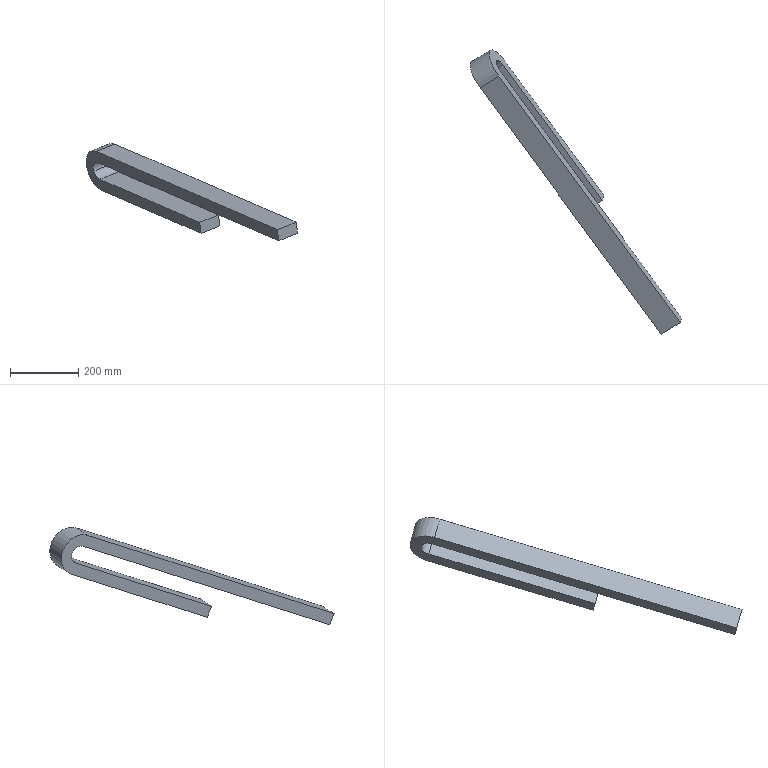Part | SolidWorks | features ExtruThin 1 | 1 solid | 12 faces | box 617.546 x 830.514 x 284.328 mm | volume 3734019 mm3 | plane 8 | cylinder 4 | commonest cylinder face diameters 54 x2 124 x2
STEP:
#1=CARTESIAN_POINT('',(136.827,-667.539,2230.426));
#2=VERTEX_POINT('',#1);
#3=CARTESIAN_POINT('',(147.549,-700.908,2255.142));
#4=VERTEX_POINT('',#3);
#5=CARTESIAN_POINT('',(150.913,-690.573,2230.426));
#6=DIRECTION('',(0.8091,0.4948,0.317));
#7=DIRECTION('',(-0.1246,-0.3828,0.9154));
#8=AXIS2_PLACEMENT_3D('',#5,#6,#7);
#9=CIRCLE('',#8,27.);
#10=EDGE_CURVE('',#2,#4,#9,.T.);
#11=ORIENTED_EDGE('',*,*,#10,.F.);
#12=CARTESIAN_POINT('',(191.847,-633.893,2251.985));
#13=VERTEX_POINT('',#12);
#14=CARTESIAN_POINT('',(136.827,-667.539,2230.426));
#15=DIRECTION('',(0.8091,0.4948,0.317));
#16=VECTOR('',#15,1000.);
#17=LINE('',#14,#16);
#18=EDGE_CURVE('',#2,#13,#17,.T.);
#19=ORIENTED_EDGE('',*,*,#18,.T.);
#20=CARTESIAN_POINT('',(202.568,-667.262,2276.7));
#21=VERTEX_POINT('',#20);
#22=CARTESIAN_POINT('',(205.933,-656.927,2251.985));
#23=DIRECTION('',(0.8091,0.4948,0.317));
#24=DIRECTION('',(-0.1246,-0.3828,0.9154));
#25=AXIS2_PLACEMENT_3D('',#22,#23,#24);
#26=CIRCLE('',#25,27.);
#27=EDGE_CURVE('',#13,#21,#26,.T.);
#28=ORIENTED_EDGE('',*,*,#27,.T.);
#29=CARTESIAN_POINT('',(147.549,-700.908,2255.142));
#30=DIRECTION('',(0.8091,0.4948,0.317));
#31=VECTOR('',#30,1000.);
#32=LINE('',#29,#31);
#33=EDGE_CURVE('',#4,#21,#32,.T.);
#34=ORIENTED_EDGE('',*,*,#33,.F.);
#35=EDGE_LOOP('',(#11,#19,#28,#34));
#36=FACE_OUTER_BOUND('',#35,.T.);
#37=CARTESIAN_POINT('',(150.913,-690.573,2230.426));
#38=DIRECTION('',(0.8091,0.4948,0.317));
#39=DIRECTION('',(-0.5217,0.8531,0.));
#40=AXIS2_PLACEMENT_3D('',#37,#38,#39);
#41=CYLINDRICAL_SURFACE('',#40,27.);
#42=ADVANCED_FACE('',(#36),#41,.F.);
#43=CARTESIAN_POINT('',(158.639,-666.841,2173.671));
#44=VERTEX_POINT('',#43);
#45=CARTESIAN_POINT('',(118.567,-637.68,2230.426));
#46=VERTEX_POINT('',#45);
#47=CARTESIAN_POINT('',(150.913,-690.573,2230.426));
#48=DIRECTION('',(0.8091,0.4948,0.317));
#49=DIRECTION('',(-0.5217,0.8531,0.));
#50=AXIS2_PLACEMENT_3D('',#47,#48,#49);
#51=CIRCLE('',#50,62.);
#52=EDGE_CURVE('',#44,#46,#51,.T.);
#53=ORIENTED_EDGE('',*,*,#52,.T.);
#54=CARTESIAN_POINT('',(173.587,-604.034,2251.985));
#55=VERTEX_POINT('',#54);
#56=CARTESIAN_POINT('',(118.567,-637.68,2230.426));
#57=DIRECTION('',(0.8091,0.4948,0.317));
#58=VECTOR('',#57,1000.);
#59=LINE('',#56,#58);
#60=EDGE_CURVE('',#46,#55,#59,.T.);
#61=ORIENTED_EDGE('',*,*,#60,.T.);
#62=CARTESIAN_POINT('',(213.659,-633.195,2195.23));
#63=VERTEX_POINT('',#62);
#64=CARTESIAN_POINT('',(205.933,-656.927,2251.985));
#65=DIRECTION('',(0.8091,0.4948,0.317));
#66=DIRECTION('',(-0.5217,0.8531,0.));
#67=AXIS2_PLACEMENT_3D('',#64,#65,#66);
#68=CIRCLE('',#67,62.);
#69=EDGE_CURVE('',#63,#55,#68,.T.);
#70=ORIENTED_EDGE('',*,*,#69,.F.);
#71=CARTESIAN_POINT('',(158.639,-666.841,2173.671));
#72=DIRECTION('',(0.8091,0.4948,0.317));
#73=VECTOR('',#72,1000.);
#74=LINE('',#71,#73);
#75=EDGE_CURVE('',#44,#63,#74,.T.);
#76=ORIENTED_EDGE('',*,*,#75,.F.);
#77=EDGE_LOOP('',(#53,#61,#70,#76));
#78=FACE_OUTER_BOUND('',#77,.T.);
#79=CARTESIAN_POINT('',(150.913,-690.573,2230.426));
#80=DIRECTION('',(0.8091,0.4948,0.317));
#81=DIRECTION('',(-0.5217,0.8531,0.));
#82=AXIS2_PLACEMENT_3D('',#79,#80,#81);
#83=CYLINDRICAL_SURFACE('',#82,62.);
#84=ADVANCED_FACE('',(#78),#83,.T.);
#85=CARTESIAN_POINT('',(198.207,-680.659,2308.739));
#86=VERTEX_POINT('',#85);
#87=CARTESIAN_POINT('',(727.663,-1399.917,2080.056));
#88=VERTEX_POINT('',#87);
#89=CARTESIAN_POINT('',(727.663,-1399.917,2080.056));
#90=DIRECTION('',(0.5743,-0.7802,-0.248));
#91=VECTOR('',#90,1000.);
#92=LINE('',#89,#91);
#93=EDGE_CURVE('',#86,#88,#92,.T.);
#94=ORIENTED_EDGE('',*,*,#93,.F.);
#95=CARTESIAN_POINT('',(143.187,-714.305,2287.181));
#96=VERTEX_POINT('',#95);
#97=CARTESIAN_POINT('',(143.187,-714.305,2287.181));
#98=DIRECTION('',(0.8091,0.4948,0.317));
#99=VECTOR('',#98,1000.);
#100=LINE('',#97,#99);
#101=EDGE_CURVE('',#96,#86,#100,.T.);
#102=ORIENTED_EDGE('',*,*,#101,.F.);
#103=CARTESIAN_POINT('',(672.643,-1433.563,2058.497));
#104=VERTEX_POINT('',#103);
#105=CARTESIAN_POINT('',(672.643,-1433.563,2058.497));
#106=DIRECTION('',(0.5743,-0.7802,-0.248));
#107=VECTOR('',#106,1000.);
#108=LINE('',#105,#107);
#109=EDGE_CURVE('',#96,#104,#108,.T.);
#110=ORIENTED_EDGE('',*,*,#109,.T.);
#111=CARTESIAN_POINT('',(672.643,-1433.563,2058.497));
#112=DIRECTION('',(0.8091,0.4948,0.317));
#113=VECTOR('',#112,1000.);
#114=LINE('',#111,#113);
#115=EDGE_CURVE('',#104,#88,#114,.T.);
#116=ORIENTED_EDGE('',*,*,#115,.T.);
#117=EDGE_LOOP('',(#94,#102,#110,#116));
#118=FACE_OUTER_BOUND('',#117,.T.);
#119=CARTESIAN_POINT('',(672.643,-1433.563,2058.497));
#120=DIRECTION('',(-0.1246,-0.3828,0.9154));
#121=DIRECTION('',(0.,-0.9226,-0.3858));
#122=AXIS2_PLACEMENT_3D('',#119,#120,#121);
#123=PLANE('',#122);
#124=ADVANCED_FACE('',(#118),#123,.T.);
#125=ORIENTED_EDGE('',*,*,#60,.F.);
#126=CARTESIAN_POINT('',(150.913,-690.573,2230.426));
#127=DIRECTION('',(0.8091,0.4948,0.317));
#128=DIRECTION('',(-0.5217,0.8531,0.));
#129=AXIS2_PLACEMENT_3D('',#126,#127,#128);
#130=CIRCLE('',#129,62.);
#131=EDGE_CURVE('',#46,#96,#130,.T.);
#132=ORIENTED_EDGE('',*,*,#131,.T.);
#133=ORIENTED_EDGE('',*,*,#101,.T.);
#134=CARTESIAN_POINT('',(205.933,-656.927,2251.985));
#135=DIRECTION('',(0.8091,0.4948,0.317));
#136=DIRECTION('',(-0.5217,0.8531,0.));
#137=AXIS2_PLACEMENT_3D('',#134,#135,#136);
#138=CIRCLE('',#137,62.);
#139=EDGE_CURVE('',#55,#86,#138,.T.);
#140=ORIENTED_EDGE('',*,*,#139,.F.);
#141=EDGE_LOOP('',(#125,#132,#133,#140));
#142=FACE_OUTER_BOUND('',#141,.T.);
#143=CARTESIAN_POINT('',(150.913,-690.573,2230.426));
#144=DIRECTION('',(0.8091,0.4948,0.317));
#145=DIRECTION('',(-0.5217,0.8531,0.));
#146=AXIS2_PLACEMENT_3D('',#143,#144,#145);
#147=CYLINDRICAL_SURFACE('',#146,62.);
#148=ADVANCED_FACE('',(#142),#147,.T.);
#149=CARTESIAN_POINT('',(504.932,-1028.885,2069.423));
#150=VERTEX_POINT('',#149);
#151=CARTESIAN_POINT('',(504.932,-1028.885,2069.423));
#152=DIRECTION('',(-0.5743,0.7802,0.248));
#153=VECTOR('',#152,1000.);
#154=LINE('',#151,#153);
#155=EDGE_CURVE('',#150,#63,#154,.T.);
#156=ORIENTED_EDGE('',*,*,#155,.F.);
#157=CARTESIAN_POINT('',(449.913,-1062.532,2047.864));
#158=VERTEX_POINT('',#157);
#159=CARTESIAN_POINT('',(449.913,-1062.532,2047.864));
#160=DIRECTION('',(0.8091,0.4948,0.317));
#161=VECTOR('',#160,1000.);
#162=LINE('',#159,#161);
#163=EDGE_CURVE('',#158,#150,#162,.T.);
#164=ORIENTED_EDGE('',*,*,#163,.F.);
#165=CARTESIAN_POINT('',(449.913,-1062.532,2047.864));
#166=DIRECTION('',(-0.5743,0.7802,0.248));
#167=VECTOR('',#166,1000.);
#168=LINE('',#165,#167);
#169=EDGE_CURVE('',#158,#44,#168,.T.);
#170=ORIENTED_EDGE('',*,*,#169,.T.);
#171=ORIENTED_EDGE('',*,*,#75,.T.);
#172=EDGE_LOOP('',(#156,#164,#170,#171));
#173=FACE_OUTER_BOUND('',#172,.T.);
#174=CARTESIAN_POINT('',(449.913,-1062.532,2047.864));
#175=DIRECTION('',(0.1246,0.3828,-0.9154));
#176=DIRECTION('',(0.,0.9226,0.3858));
#177=AXIS2_PLACEMENT_3D('',#174,#175,#176);
#178=PLANE('',#177);
#179=ADVANCED_FACE('',(#173),#178,.T.);
#180=CARTESIAN_POINT('',(500.571,-1042.283,2101.462));
#181=VERTEX_POINT('',#180);
#182=CARTESIAN_POINT('',(504.932,-1028.885,2069.423));
#183=DIRECTION('',(-0.1246,-0.3828,0.9154));
#184=VECTOR('',#183,1000.);
#185=LINE('',#182,#184);
#186=EDGE_CURVE('',#150,#181,#185,.T.);
#187=ORIENTED_EDGE('',*,*,#186,.T.);
#188=CARTESIAN_POINT('',(445.551,-1075.929,2079.903));
#189=VERTEX_POINT('',#188);
#190=CARTESIAN_POINT('',(445.551,-1075.929,2079.903));
#191=DIRECTION('',(0.8091,0.4948,0.317));
#192=VECTOR('',#191,1000.);
#193=LINE('',#190,#192);
#194=EDGE_CURVE('',#189,#181,#193,.T.);
#195=ORIENTED_EDGE('',*,*,#194,.F.);
#196=CARTESIAN_POINT('',(449.913,-1062.532,2047.864));
#197=DIRECTION('',(-0.1246,-0.3828,0.9154));
#198=VECTOR('',#197,1000.);
#199=LINE('',#196,#198);
#200=EDGE_CURVE('',#158,#189,#199,.T.);
#201=ORIENTED_EDGE('',*,*,#200,.F.);
#202=ORIENTED_EDGE('',*,*,#163,.T.);
#203=EDGE_LOOP('',(#187,#195,#201,#202));
#204=FACE_OUTER_BOUND('',#203,.T.);
#205=CARTESIAN_POINT('',(449.913,-1062.532,2047.864));
#206=DIRECTION('',(-0.5743,0.7802,0.248));
#207=DIRECTION('',(-0.8053,-0.5928,0.));
#208=AXIS2_PLACEMENT_3D('',#205,#206,#207);
#209=PLANE('',#208);
#210=ADVANCED_FACE('',(#204),#209,.F.);
#211=CARTESIAN_POINT('',(209.297,-646.592,2227.269));
#212=VERTEX_POINT('',#211);
#213=CARTESIAN_POINT('',(500.571,-1042.283,2101.462));
#214=DIRECTION('',(-0.5743,0.7802,0.248));
#215=VECTOR('',#214,1000.);
#216=LINE('',#213,#215);
#217=EDGE_CURVE('',#181,#212,#216,.T.);
#218=ORIENTED_EDGE('',*,*,#217,.T.);
#219=CARTESIAN_POINT('',(154.278,-680.239,2205.71));
#220=VERTEX_POINT('',#219);
#221=CARTESIAN_POINT('',(154.278,-680.239,2205.71));
#222=DIRECTION('',(0.8091,0.4948,0.317));
#223=VECTOR('',#222,1000.);
#224=LINE('',#221,#223);
#225=EDGE_CURVE('',#220,#212,#224,.T.);
#226=ORIENTED_EDGE('',*,*,#225,.F.);
#227=CARTESIAN_POINT('',(445.551,-1075.929,2079.903));
#228=DIRECTION('',(-0.5743,0.7802,0.248));
#229=VECTOR('',#228,1000.);
#230=LINE('',#227,#229);
#231=EDGE_CURVE('',#189,#220,#230,.T.);
#232=ORIENTED_EDGE('',*,*,#231,.F.);
#233=ORIENTED_EDGE('',*,*,#194,.T.);
#234=EDGE_LOOP('',(#218,#226,#232,#233));
#235=FACE_OUTER_BOUND('',#234,.T.);
#236=CARTESIAN_POINT('',(445.551,-1075.929,2079.903));
#237=DIRECTION('',(0.1246,0.3828,-0.9154));
#238=DIRECTION('',(0.,0.9226,0.3858));
#239=AXIS2_PLACEMENT_3D('',#236,#237,#238);
#240=PLANE('',#239);
#241=ADVANCED_FACE('',(#235),#240,.F.);
#242=ORIENTED_EDGE('',*,*,#18,.F.);
#243=CARTESIAN_POINT('',(150.913,-690.573,2230.426));
#244=DIRECTION('',(0.8091,0.4948,0.317));
#245=DIRECTION('',(-0.1246,-0.3828,0.9154));
#246=AXIS2_PLACEMENT_3D('',#243,#244,#245);
#247=CIRCLE('',#246,27.);
#248=EDGE_CURVE('',#220,#2,#247,.T.);
#249=ORIENTED_EDGE('',*,*,#248,.F.);
#250=ORIENTED_EDGE('',*,*,#225,.T.);
#251=CARTESIAN_POINT('',(205.933,-656.927,2251.985));
#252=DIRECTION('',(0.8091,0.4948,0.317));
#253=DIRECTION('',(-0.1246,-0.3828,0.9154));
#254=AXIS2_PLACEMENT_3D('',#251,#252,#253);
#255=CIRCLE('',#254,27.);
#256=EDGE_CURVE('',#212,#13,#255,.T.);
#257=ORIENTED_EDGE('',*,*,#256,.T.);
#258=EDGE_LOOP('',(#242,#249,#250,#257));
#259=FACE_OUTER_BOUND('',#258,.T.);
#260=CARTESIAN_POINT('',(150.913,-690.573,2230.426));
#261=DIRECTION('',(0.8091,0.4948,0.317));
#262=DIRECTION('',(-0.5217,0.8531,0.));
#263=AXIS2_PLACEMENT_3D('',#260,#261,#262);
#264=CYLINDRICAL_SURFACE('',#263,27.);
#265=ADVANCED_FACE('',(#259),#264,.F.);
#266=CARTESIAN_POINT('',(732.024,-1386.52,2048.017));
#267=VERTEX_POINT('',#266);
#268=CARTESIAN_POINT('',(732.024,-1386.52,2048.017));
#269=DIRECTION('',(0.5743,-0.7802,-0.248));
#270=VECTOR('',#269,1000.);
#271=LINE('',#268,#270);
#272=EDGE_CURVE('',#21,#267,#271,.T.);
#273=ORIENTED_EDGE('',*,*,#272,.T.);
#274=CARTESIAN_POINT('',(677.005,-1420.166,2026.458));
#275=VERTEX_POINT('',#274);
#276=CARTESIAN_POINT('',(677.005,-1420.166,2026.458));
#277=DIRECTION('',(0.8091,0.4948,0.317));
#278=VECTOR('',#277,1000.);
#279=LINE('',#276,#278);
#280=EDGE_CURVE('',#275,#267,#279,.T.);
#281=ORIENTED_EDGE('',*,*,#280,.F.);
#282=CARTESIAN_POINT('',(677.005,-1420.166,2026.458));
#283=DIRECTION('',(0.5743,-0.7802,-0.248));
#284=VECTOR('',#283,1000.);
#285=LINE('',#282,#284);
#286=EDGE_CURVE('',#4,#275,#285,.T.);
#287=ORIENTED_EDGE('',*,*,#286,.F.);
#288=ORIENTED_EDGE('',*,*,#33,.T.);
#289=EDGE_LOOP('',(#273,#281,#287,#288));
#290=FACE_OUTER_BOUND('',#289,.T.);
#291=CARTESIAN_POINT('',(677.005,-1420.166,2026.458));
#292=DIRECTION('',(-0.1246,-0.3828,0.9154));
#293=DIRECTION('',(0.,-0.9226,-0.3858));
#294=AXIS2_PLACEMENT_3D('',#291,#292,#293);
#295=PLANE('',#294);
#296=ADVANCED_FACE('',(#290),#295,.F.);
#297=CARTESIAN_POINT('',(732.024,-1386.52,2048.017));
#298=DIRECTION('',(-0.1246,-0.3828,0.9154));
#299=VECTOR('',#298,1000.);
#300=LINE('',#297,#299);
#301=EDGE_CURVE('',#267,#88,#300,.T.);
#302=ORIENTED_EDGE('',*,*,#301,.T.);
#303=ORIENTED_EDGE('',*,*,#115,.F.);
#304=CARTESIAN_POINT('',(677.005,-1420.166,2026.458));
#305=DIRECTION('',(-0.1246,-0.3828,0.9154));
#306=VECTOR('',#305,1000.);
#307=LINE('',#304,#306);
#308=EDGE_CURVE('',#275,#104,#307,.T.);
#309=ORIENTED_EDGE('',*,*,#308,.F.);
#310=ORIENTED_EDGE('',*,*,#280,.T.);
#311=EDGE_LOOP('',(#302,#303,#309,#310));
#312=FACE_OUTER_BOUND('',#311,.T.);
#313=CARTESIAN_POINT('',(677.005,-1420.166,2026.458));
#314=DIRECTION('',(-0.5743,0.7802,0.248));
#315=DIRECTION('',(-0.8053,-0.5928,0.));
#316=AXIS2_PLACEMENT_3D('',#313,#314,#315);
#317=PLANE('',#316);
#318=ADVANCED_FACE('',(#312),#317,.F.);
#319=ORIENTED_EDGE('',*,*,#109,.F.);
#320=ORIENTED_EDGE('',*,*,#131,.F.);
#321=ORIENTED_EDGE('',*,*,#52,.F.);
#322=ORIENTED_EDGE('',*,*,#169,.F.);
#323=ORIENTED_EDGE('',*,*,#200,.T.);
#324=ORIENTED_EDGE('',*,*,#231,.T.);
#325=ORIENTED_EDGE('',*,*,#248,.T.);
#326=ORIENTED_EDGE('',*,*,#10,.T.);
#327=ORIENTED_EDGE('',*,*,#286,.T.);
#328=ORIENTED_EDGE('',*,*,#308,.T.);
#329=EDGE_LOOP('',(#319,#320,#321,#322,#323,#324,#325,#326,#327,#328));
#330=FACE_OUTER_BOUND('',#329,.T.);
#331=CARTESIAN_POINT('',(150.913,-690.573,2230.426));
#332=DIRECTION('',(0.8091,0.4948,0.317));
#333=DIRECTION('',(-0.1246,-0.3828,0.9154));
#334=AXIS2_PLACEMENT_3D('',#331,#332,#333);
#335=PLANE('',#334);
#336=ADVANCED_FACE('',(#330),#335,.F.);
#337=ORIENTED_EDGE('',*,*,#93,.T.);
#338=ORIENTED_EDGE('',*,*,#301,.F.);
#339=ORIENTED_EDGE('',*,*,#272,.F.);
#340=ORIENTED_EDGE('',*,*,#27,.F.);
#341=ORIENTED_EDGE('',*,*,#256,.F.);
#342=ORIENTED_EDGE('',*,*,#217,.F.);
#343=ORIENTED_EDGE('',*,*,#186,.F.);
#344=ORIENTED_EDGE('',*,*,#155,.T.);
#345=ORIENTED_EDGE('',*,*,#69,.T.);
#346=ORIENTED_EDGE('',*,*,#139,.T.);
#347=EDGE_LOOP('',(#337,#338,#339,#340,#341,#342,#343,#344,#345,#346));
#348=FACE_OUTER_BOUND('',#347,.T.);
#349=CARTESIAN_POINT('',(205.933,-656.927,2251.985));
#350=DIRECTION('',(0.8091,0.4948,0.317));
#351=DIRECTION('',(-0.1246,-0.3828,0.9154));
#352=AXIS2_PLACEMENT_3D('',#349,#350,#351);
#353=PLANE('',#352);
#354=ADVANCED_FACE('',(#348),#353,.T.);
#355=CLOSED_SHELL('',(#42,#84,#124,#148,#179,#210,#241,#265,#296,#318,#336,#354));
#356=MANIFOLD_SOLID_BREP('',#355);
#357=CARTESIAN_POINT('',(0.,0.,0.));
#358=DIRECTION('',(0.,0.,1.));
#359=DIRECTION('',(1.,0.,0.));
#360=AXIS2_PLACEMENT_3D('',#357,#358,#359);
#361=(LENGTH_UNIT()NAMED_UNIT(*)SI_UNIT(.MILLI.,.METRE.));
#362=UNCERTAINTY_MEASURE_WITH_UNIT(LENGTH_MEASURE(0.00001),#361,'','');
#363=(NAMED_UNIT(*)PLANE_ANGLE_UNIT()SI_UNIT($,.RADIAN.));
#364=(NAMED_UNIT(*)SI_UNIT($,.STERADIAN.)SOLID_ANGLE_UNIT());
#365=(GEOMETRIC_REPRESENTATION_CONTEXT(3)GLOBAL_UNCERTAINTY_ASSIGNED_CONTEXT((#362))GLOBAL_UNIT_ASSIGNED_CONTEXT((#361,#363,#364))REPRESENTATION_CONTEXT('',''));
#366=ADVANCED_BREP_SHAPE_REPRESENTATION('',(#356,#360),#365);